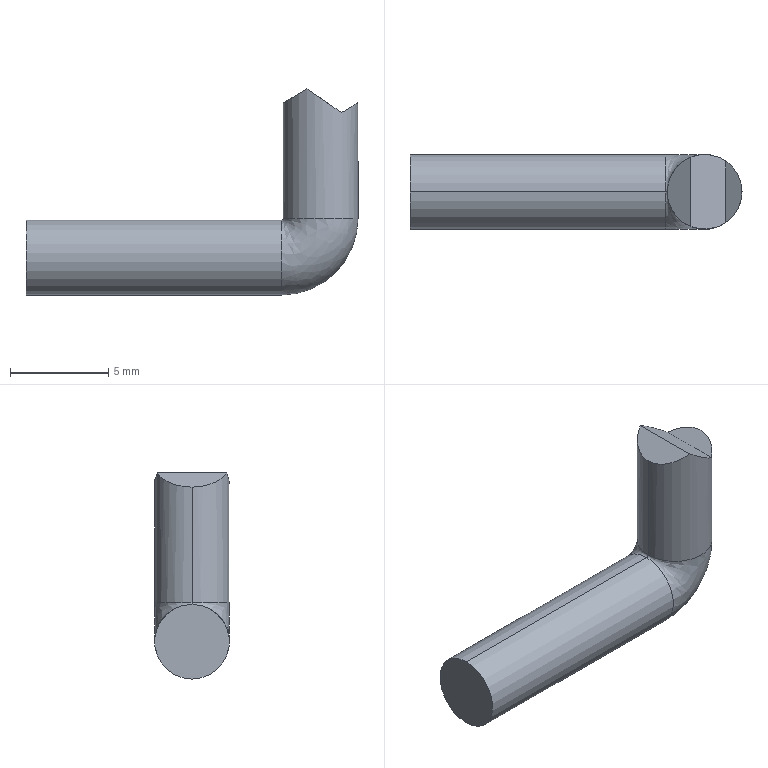Part | SolidWorks | features BaseBody 1 | 1 solid | 10 faces | box 16.9 x 3.8 x 10.488 mm | volume 251.226 mm3 | cylinder 4 | plane 4 | spline 2 | commonest cylinder face diameters 3.8 x4
STEP:
#1=CARTESIAN_POINT('',(-2.,-0.5,-18.1));
#2=VERTEX_POINT('',#1);
#3=CARTESIAN_POINT('',(-2.,-0.5,-21.9));
#4=VERTEX_POINT('',#3);
#5=CARTESIAN_POINT('',(-2.,-0.5,-20.));
#6=DIRECTION('',(-1.,0.,0.));
#7=DIRECTION('',(0.,0.,1.));
#8=AXIS2_PLACEMENT_3D('',#5,#6,#7);
#9=CIRCLE('',#8,1.9);
#10=EDGE_CURVE('',#2,#4,#9,.T.);
#11=ORIENTED_EDGE('',*,*,#10,.T.);
#12=CARTESIAN_POINT('',(-15.,-0.5,-21.9));
#13=VERTEX_POINT('',#12);
#14=CARTESIAN_POINT('',(-2.,-0.5,-21.9));
#15=DIRECTION('',(-1.,0.,0.));
#16=VECTOR('',#15,1000.);
#17=LINE('',#14,#16);
#18=EDGE_CURVE('',#4,#13,#17,.T.);
#19=ORIENTED_EDGE('',*,*,#18,.T.);
#20=CARTESIAN_POINT('',(-15.,-0.5,-18.1));
#21=VERTEX_POINT('',#20);
#22=CARTESIAN_POINT('',(-15.,-0.5,-20.));
#23=DIRECTION('',(1.,0.,0.));
#24=DIRECTION('',(0.,0.,1.));
#25=AXIS2_PLACEMENT_3D('',#22,#23,#24);
#26=CIRCLE('',#25,1.9);
#27=EDGE_CURVE('',#13,#21,#26,.T.);
#28=ORIENTED_EDGE('',*,*,#27,.T.);
#29=CARTESIAN_POINT('',(-2.,-0.5,-18.1));
#30=DIRECTION('',(-1.,0.,0.));
#31=VECTOR('',#30,1000.);
#32=LINE('',#29,#31);
#33=EDGE_CURVE('',#2,#21,#32,.T.);
#34=ORIENTED_EDGE('',*,*,#33,.F.);
#35=EDGE_LOOP('',(#11,#19,#28,#34));
#36=FACE_OUTER_BOUND('',#35,.T.);
#37=CARTESIAN_POINT('',(-2.,-0.5,-20.));
#38=DIRECTION('',(-1.,0.,0.));
#39=DIRECTION('',(0.,0.,1.));
#40=AXIS2_PLACEMENT_3D('',#37,#38,#39);
#41=CYLINDRICAL_SURFACE('',#40,1.9);
#42=ADVANCED_FACE('',(#36),#41,.T.);
#43=CARTESIAN_POINT('',(1.9,-0.5,-18.));
#44=VERTEX_POINT('',#43);
#45=CARTESIAN_POINT('',(-1.9,-0.5,-18.));
#46=VERTEX_POINT('',#45);
#47=CARTESIAN_POINT('',(0.,-0.5,-18.));
#48=DIRECTION('',(0.,0.,-1.));
#49=DIRECTION('',(1.,0.,0.));
#50=AXIS2_PLACEMENT_3D('',#47,#48,#49);
#51=CIRCLE('',#50,1.9);
#52=EDGE_CURVE('',#44,#46,#51,.T.);
#53=ORIENTED_EDGE('',*,*,#52,.T.);
#54=CARTESIAN_POINT('',(-2.,-0.5,-18.));
#55=DIRECTION('',(0.,1.,0.));
#56=DIRECTION('',(0.,0.,1.));
#57=AXIS2_PLACEMENT_3D('',#54,#55,#56);
#58=CIRCLE('',#57,0.1);
#59=EDGE_CURVE('',#46,#2,#58,.T.);
#60=ORIENTED_EDGE('',*,*,#59,.T.);
#61=CARTESIAN_POINT('',(-2.,-0.5,-20.));
#62=DIRECTION('',(-1.,0.,0.));
#63=DIRECTION('',(0.,0.,1.));
#64=AXIS2_PLACEMENT_3D('',#61,#62,#63);
#65=CIRCLE('',#64,1.9);
#66=EDGE_CURVE('',#4,#2,#65,.T.);
#67=ORIENTED_EDGE('',*,*,#66,.F.);
#68=CARTESIAN_POINT('',(-2.,-0.5,-18.));
#69=DIRECTION('',(0.,1.,0.));
#70=DIRECTION('',(0.,0.,1.));
#71=AXIS2_PLACEMENT_3D('',#68,#69,#70);
#72=CIRCLE('',#71,3.9);
#73=EDGE_CURVE('',#44,#4,#72,.T.);
#74=ORIENTED_EDGE('',*,*,#73,.F.);
#75=EDGE_LOOP('',(#53,#60,#67,#74));
#76=FACE_OUTER_BOUND('',#75,.T.);
#77=CARTESIAN_POINT('',(1.9,-0.5,-18.));
#78=CARTESIAN_POINT('',(1.9,-0.5,-20.285));
#79=CARTESIAN_POINT('',(0.2846,-0.5,-21.9));
#80=CARTESIAN_POINT('',(-2.,-0.5,-21.9));
#81=CARTESIAN_POINT('',(1.9,-4.3,-18.));
#82=CARTESIAN_POINT('',(1.9,-4.3,-20.285));
#83=CARTESIAN_POINT('',(0.2846,-4.3,-21.9));
#84=CARTESIAN_POINT('',(-2.,-4.3,-21.9));
#85=CARTESIAN_POINT('',(-1.9,-4.3,-18.));
#86=CARTESIAN_POINT('',(-1.9,-4.3,-18.059));
#87=CARTESIAN_POINT('',(-1.941,-4.3,-18.1));
#88=CARTESIAN_POINT('',(-2.,-4.3,-18.1));
#89=CARTESIAN_POINT('',(-1.9,-0.5,-18.));
#90=CARTESIAN_POINT('',(-1.9,-0.5,-18.059));
#91=CARTESIAN_POINT('',(-1.941,-0.5,-18.1));
#92=CARTESIAN_POINT('',(-2.,-0.5,-18.1));
#93=(BOUNDED_SURFACE()B_SPLINE_SURFACE(3,3,((#77,#78,#79,#80),(#81,#82,#83,#84),(#85,#86,#87,#88),(#89,#90,#91,#92)),.UNSPECIFIED.,.F.,.F.,.F.)B_SPLINE_SURFACE_WITH_KNOTS((4,4),(4,4),(0.,1.),(0.,1.),.UNSPECIFIED.)GEOMETRIC_REPRESENTATION_ITEM()RATIONAL_B_SPLINE_SURFACE(((1.,0.8047,0.8047,1.),(0.3333,0.2682,0.2682,0.3333),(0.3333,0.2682,0.2682,0.3333),(1.,0.8047,0.8047,1.)))REPRESENTATION_ITEM('')SURFACE());
#94=ADVANCED_FACE('',(#76),#93,.T.);
#95=CARTESIAN_POINT('',(1.068,1.071,-12.617));
#96=VERTEX_POINT('',#95);
#97=CARTESIAN_POINT('',(1.9,-0.5,-12.12));
#98=VERTEX_POINT('',#97);
#99=CARTESIAN_POINT('',(1.068,1.071,-12.617));
#100=CARTESIAN_POINT('',(1.599,0.7103,-12.3));
#101=CARTESIAN_POINT('',(1.9,0.1425,-12.12));
#102=CARTESIAN_POINT('',(1.9,-0.5,-12.12));
#103=(BOUNDED_CURVE()B_SPLINE_CURVE(3,(#99,#100,#101,#102),.UNSPECIFIED.,.F.,.F.)B_SPLINE_CURVE_WITH_KNOTS((4,4),(2.168,3.142),.UNSPECIFIED.)CURVE()GEOMETRIC_REPRESENTATION_ITEM()RATIONAL_B_SPLINE_CURVE((1.,0.9225,0.9225,1.))REPRESENTATION_ITEM(''));
#104=EDGE_CURVE('',#96,#98,#103,.T.);
#105=ORIENTED_EDGE('',*,*,#104,.T.);
#106=CARTESIAN_POINT('',(1.9,-0.5,0.));
#107=DIRECTION('',(0.,0.,-1.));
#108=VECTOR('',#107,1000.);
#109=LINE('',#106,#108);
#110=EDGE_CURVE('',#98,#44,#109,.T.);
#111=ORIENTED_EDGE('',*,*,#110,.T.);
#112=CARTESIAN_POINT('',(0.,-0.5,-18.));
#113=DIRECTION('',(0.,0.,-1.));
#114=DIRECTION('',(1.,0.,0.));
#115=AXIS2_PLACEMENT_3D('',#112,#113,#114);
#116=CIRCLE('',#115,1.9);
#117=EDGE_CURVE('',#46,#44,#116,.T.);
#118=ORIENTED_EDGE('',*,*,#117,.F.);
#119=CARTESIAN_POINT('',(-1.9,-0.5,-12.129));
#120=VERTEX_POINT('',#119);
#121=CARTESIAN_POINT('',(-1.9,-0.5,0.));
#122=DIRECTION('',(0.,0.,-1.));
#123=VECTOR('',#122,1000.);
#124=LINE('',#121,#123);
#125=EDGE_CURVE('',#120,#46,#124,.T.);
#126=ORIENTED_EDGE('',*,*,#125,.F.);
#127=CARTESIAN_POINT('',(-0.6971,1.267,-11.412));
#128=VERTEX_POINT('',#127);
#129=CARTESIAN_POINT('',(-1.9,-0.5,-12.129));
#130=CARTESIAN_POINT('',(-1.9,0.3057,-12.129));
#131=CARTESIAN_POINT('',(-1.447,0.9719,-11.859));
#132=CARTESIAN_POINT('',(-0.6971,1.267,-11.412));
#133=(BOUNDED_CURVE()B_SPLINE_CURVE(3,(#129,#130,#131,#132),.UNSPECIFIED.,.F.,.F.)B_SPLINE_CURVE_WITH_KNOTS((4,4),(0.,1.195),.UNSPECIFIED.)CURVE()GEOMETRIC_REPRESENTATION_ITEM()RATIONAL_B_SPLINE_CURVE((1.,0.8845,0.8845,1.))REPRESENTATION_ITEM(''));
#134=EDGE_CURVE('',#120,#128,#133,.T.);
#135=ORIENTED_EDGE('',*,*,#134,.T.);
#136=CARTESIAN_POINT('',(-0.6971,1.267,-11.412));
#137=CARTESIAN_POINT('',(-0.1003,1.503,-11.819));
#138=CARTESIAN_POINT('',(0.5373,1.432,-12.254));
#139=CARTESIAN_POINT('',(1.068,1.071,-12.617));
#140=(BOUNDED_CURVE()B_SPLINE_CURVE(3,(#136,#137,#138,#139),.UNSPECIFIED.,.F.,.F.)B_SPLINE_CURVE_WITH_KNOTS((4,4),(4.337,5.309),.UNSPECIFIED.)CURVE()GEOMETRIC_REPRESENTATION_ITEM()RATIONAL_B_SPLINE_CURVE((1.,0.9227,0.9227,1.))REPRESENTATION_ITEM(''));
#141=EDGE_CURVE('',#128,#96,#140,.T.);
#142=ORIENTED_EDGE('',*,*,#141,.T.);
#143=EDGE_LOOP('',(#105,#111,#118,#126,#135,#142));
#144=FACE_OUTER_BOUND('',#143,.T.);
#145=CARTESIAN_POINT('',(0.,-0.5,0.));
#146=DIRECTION('',(0.,0.,-1.));
#147=DIRECTION('',(-1.,0.,0.));
#148=AXIS2_PLACEMENT_3D('',#145,#146,#147);
#149=CYLINDRICAL_SURFACE('',#148,1.9);
#150=ADVANCED_FACE('',(#144),#149,.T.);
#151=ORIENTED_EDGE('',*,*,#18,.F.);
#152=ORIENTED_EDGE('',*,*,#66,.T.);
#153=ORIENTED_EDGE('',*,*,#33,.T.);
#154=CARTESIAN_POINT('',(-15.,-0.5,-20.));
#155=DIRECTION('',(1.,0.,0.));
#156=DIRECTION('',(0.,0.,1.));
#157=AXIS2_PLACEMENT_3D('',#154,#155,#156);
#158=CIRCLE('',#157,1.9);
#159=EDGE_CURVE('',#21,#13,#158,.T.);
#160=ORIENTED_EDGE('',*,*,#159,.T.);
#161=EDGE_LOOP('',(#151,#152,#153,#160));
#162=FACE_OUTER_BOUND('',#161,.T.);
#163=CARTESIAN_POINT('',(-2.,-0.5,-20.));
#164=DIRECTION('',(-1.,0.,0.));
#165=DIRECTION('',(0.,0.,1.));
#166=AXIS2_PLACEMENT_3D('',#163,#164,#165);
#167=CYLINDRICAL_SURFACE('',#166,1.9);
#168=ADVANCED_FACE('',(#162),#167,.T.);
#169=ORIENTED_EDGE('',*,*,#59,.F.);
#170=ORIENTED_EDGE('',*,*,#117,.T.);
#171=ORIENTED_EDGE('',*,*,#73,.T.);
#172=ORIENTED_EDGE('',*,*,#10,.F.);
#173=EDGE_LOOP('',(#169,#170,#171,#172));
#174=FACE_OUTER_BOUND('',#173,.T.);
#175=CARTESIAN_POINT('',(-1.9,-0.5,-18.));
#176=CARTESIAN_POINT('',(-1.9,-0.5,-18.059));
#177=CARTESIAN_POINT('',(-1.941,-0.5,-18.1));
#178=CARTESIAN_POINT('',(-2.,-0.5,-18.1));
#179=CARTESIAN_POINT('',(-1.9,3.3,-18.));
#180=CARTESIAN_POINT('',(-1.9,3.3,-18.059));
#181=CARTESIAN_POINT('',(-1.941,3.3,-18.1));
#182=CARTESIAN_POINT('',(-2.,3.3,-18.1));
#183=CARTESIAN_POINT('',(1.9,3.3,-18.));
#184=CARTESIAN_POINT('',(1.9,3.3,-20.285));
#185=CARTESIAN_POINT('',(0.2846,3.3,-21.9));
#186=CARTESIAN_POINT('',(-2.,3.3,-21.9));
#187=CARTESIAN_POINT('',(1.9,-0.5,-18.));
#188=CARTESIAN_POINT('',(1.9,-0.5,-20.285));
#189=CARTESIAN_POINT('',(0.2846,-0.5,-21.9));
#190=CARTESIAN_POINT('',(-2.,-0.5,-21.9));
#191=(BOUNDED_SURFACE()B_SPLINE_SURFACE(3,3,((#175,#176,#177,#178),(#179,#180,#181,#182),(#183,#184,#185,#186),(#187,#188,#189,#190)),.UNSPECIFIED.,.F.,.F.,.F.)B_SPLINE_SURFACE_WITH_KNOTS((4,4),(4,4),(0.,1.),(0.,1.),.UNSPECIFIED.)GEOMETRIC_REPRESENTATION_ITEM()RATIONAL_B_SPLINE_SURFACE(((1.,0.8047,0.8047,1.),(0.3333,0.2682,0.2682,0.3333),(0.3333,0.2682,0.2682,0.3333),(1.,0.8047,0.8047,1.)))REPRESENTATION_ITEM('')SURFACE());
#192=ADVANCED_FACE('',(#174),#191,.T.);
#193=ORIENTED_EDGE('',*,*,#159,.F.);
#194=ORIENTED_EDGE('',*,*,#27,.F.);
#195=EDGE_LOOP('',(#193,#194));
#196=FACE_OUTER_BOUND('',#195,.T.);
#197=CARTESIAN_POINT('',(-15.,-0.5,-20.));
#198=DIRECTION('',(-1.,0.,0.));
#199=DIRECTION('',(0.,0.,1.));
#200=AXIS2_PLACEMENT_3D('',#197,#198,#199);
#201=PLANE('',#200);
#202=ADVANCED_FACE('',(#196),#201,.T.);
#203=ORIENTED_EDGE('',*,*,#110,.F.);
#204=CARTESIAN_POINT('',(1.068,-2.071,-12.617));
#205=VERTEX_POINT('',#204);
#206=CARTESIAN_POINT('',(1.9,-0.5,-12.12));
#207=CARTESIAN_POINT('',(1.9,-1.143,-12.12));
#208=CARTESIAN_POINT('',(1.599,-1.71,-12.3));
#209=CARTESIAN_POINT('',(1.068,-2.071,-12.617));
#210=(BOUNDED_CURVE()B_SPLINE_CURVE(3,(#206,#207,#208,#209),.UNSPECIFIED.,.F.,.F.)B_SPLINE_CURVE_WITH_KNOTS((4,4),(3.142,4.116),.UNSPECIFIED.)CURVE()GEOMETRIC_REPRESENTATION_ITEM()RATIONAL_B_SPLINE_CURVE((1.,0.9225,0.9225,1.))REPRESENTATION_ITEM(''));
#211=EDGE_CURVE('',#98,#205,#210,.T.);
#212=ORIENTED_EDGE('',*,*,#211,.T.);
#213=CARTESIAN_POINT('',(-0.6971,-2.267,-11.412));
#214=VERTEX_POINT('',#213);
#215=CARTESIAN_POINT('',(1.068,-2.071,-12.617));
#216=CARTESIAN_POINT('',(0.5373,-2.432,-12.254));
#217=CARTESIAN_POINT('',(-0.1003,-2.503,-11.819));
#218=CARTESIAN_POINT('',(-0.6971,-2.267,-11.412));
#219=(BOUNDED_CURVE()B_SPLINE_CURVE(3,(#215,#216,#217,#218),.UNSPECIFIED.,.F.,.F.)B_SPLINE_CURVE_WITH_KNOTS((4,4),(0.9739,1.946),.UNSPECIFIED.)CURVE()GEOMETRIC_REPRESENTATION_ITEM()RATIONAL_B_SPLINE_CURVE((1.,0.9227,0.9227,1.))REPRESENTATION_ITEM(''));
#220=EDGE_CURVE('',#205,#214,#219,.T.);
#221=ORIENTED_EDGE('',*,*,#220,.T.);
#222=CARTESIAN_POINT('',(-0.6971,-2.267,-11.412));
#223=CARTESIAN_POINT('',(-1.447,-1.972,-11.859));
#224=CARTESIAN_POINT('',(-1.9,-1.306,-12.129));
#225=CARTESIAN_POINT('',(-1.9,-0.5,-12.129));
#226=(BOUNDED_CURVE()B_SPLINE_CURVE(3,(#222,#223,#224,#225),.UNSPECIFIED.,.F.,.F.)B_SPLINE_CURVE_WITH_KNOTS((4,4),(5.088,6.283),.UNSPECIFIED.)CURVE()GEOMETRIC_REPRESENTATION_ITEM()RATIONAL_B_SPLINE_CURVE((1.,0.8845,0.8845,1.))REPRESENTATION_ITEM(''));
#227=EDGE_CURVE('',#214,#120,#226,.T.);
#228=ORIENTED_EDGE('',*,*,#227,.T.);
#229=ORIENTED_EDGE('',*,*,#125,.T.);
#230=ORIENTED_EDGE('',*,*,#52,.F.);
#231=EDGE_LOOP('',(#203,#212,#221,#228,#229,#230));
#232=FACE_OUTER_BOUND('',#231,.T.);
#233=CARTESIAN_POINT('',(0.,-0.5,0.));
#234=DIRECTION('',(0.,0.,-1.));
#235=DIRECTION('',(-1.,0.,0.));
#236=AXIS2_PLACEMENT_3D('',#233,#234,#235);
#237=CYLINDRICAL_SURFACE('',#236,1.9);
#238=ADVANCED_FACE('',(#232),#237,.T.);
#239=ORIENTED_EDGE('',*,*,#104,.F.);
#240=CARTESIAN_POINT('',(1.068,6.15,-12.617));
#241=DIRECTION('',(0.,1.,0.));
#242=VECTOR('',#241,1000.);
#243=LINE('',#240,#242);
#244=EDGE_CURVE('',#205,#96,#243,.T.);
#245=ORIENTED_EDGE('',*,*,#244,.F.);
#246=ORIENTED_EDGE('',*,*,#211,.F.);
#247=EDGE_LOOP('',(#239,#245,#246));
#248=FACE_OUTER_BOUND('',#247,.T.);
#249=CARTESIAN_POINT('',(1.068,6.15,-12.617));
#250=DIRECTION('',(0.5122,0.,-0.8589));
#251=DIRECTION('',(-0.8589,0.,-0.5122));
#252=AXIS2_PLACEMENT_3D('',#249,#250,#251);
#253=PLANE('',#252);
#254=ADVANCED_FACE('',(#248),#253,.F.);
#255=CARTESIAN_POINT('',(-0.6971,6.15,-11.412));
#256=DIRECTION('',(0.,1.,0.));
#257=VECTOR('',#256,1000.);
#258=LINE('',#255,#257);
#259=EDGE_CURVE('',#214,#128,#258,.T.);
#260=ORIENTED_EDGE('',*,*,#259,.F.);
#261=ORIENTED_EDGE('',*,*,#220,.F.);
#262=ORIENTED_EDGE('',*,*,#244,.T.);
#263=ORIENTED_EDGE('',*,*,#141,.F.);
#264=EDGE_LOOP('',(#260,#261,#262,#263));
#265=FACE_OUTER_BOUND('',#264,.T.);
#266=CARTESIAN_POINT('',(-0.6971,6.15,-11.412));
#267=DIRECTION('',(-0.5638,0.,-0.8259));
#268=DIRECTION('',(-0.8259,0.,0.5638));
#269=AXIS2_PLACEMENT_3D('',#266,#267,#268);
#270=PLANE('',#269);
#271=ADVANCED_FACE('',(#265),#270,.F.);
#272=ORIENTED_EDGE('',*,*,#259,.T.);
#273=ORIENTED_EDGE('',*,*,#134,.F.);
#274=ORIENTED_EDGE('',*,*,#227,.F.);
#275=EDGE_LOOP('',(#272,#273,#274));
#276=FACE_OUTER_BOUND('',#275,.T.);
#277=CARTESIAN_POINT('',(-2.986,6.15,-12.777));
#278=DIRECTION('',(0.5122,0.,-0.8589));
#279=DIRECTION('',(-0.8589,0.,-0.5122));
#280=AXIS2_PLACEMENT_3D('',#277,#278,#279);
#281=PLANE('',#280);
#282=ADVANCED_FACE('',(#276),#281,.F.);
#283=CLOSED_SHELL('',(#42,#94,#150,#168,#192,#202,#238,#254,#271,#282));
#284=MANIFOLD_SOLID_BREP('',#283);
#285=CARTESIAN_POINT('',(0.,0.,0.));
#286=DIRECTION('',(0.,0.,1.));
#287=DIRECTION('',(1.,0.,0.));
#288=AXIS2_PLACEMENT_3D('',#285,#286,#287);
#289=(LENGTH_UNIT()NAMED_UNIT(*)SI_UNIT(.MILLI.,.METRE.));
#290=UNCERTAINTY_MEASURE_WITH_UNIT(LENGTH_MEASURE(0.00001),#289,'','');
#291=(NAMED_UNIT(*)PLANE_ANGLE_UNIT()SI_UNIT($,.RADIAN.));
#292=(NAMED_UNIT(*)SI_UNIT($,.STERADIAN.)SOLID_ANGLE_UNIT());
#293=(GEOMETRIC_REPRESENTATION_CONTEXT(3)GLOBAL_UNCERTAINTY_ASSIGNED_CONTEXT((#290))GLOBAL_UNIT_ASSIGNED_CONTEXT((#289,#291,#292))REPRESENTATION_CONTEXT('',''));
#294=ADVANCED_BREP_SHAPE_REPRESENTATION('',(#284,#288),#293);